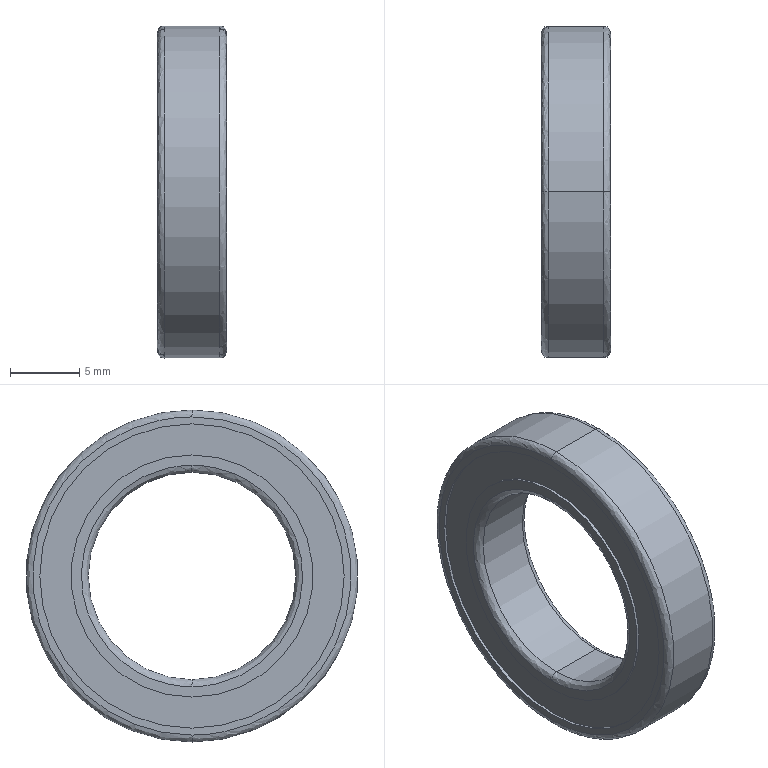Part | STEP file | Bearing 6802zz | 1 solid | 26 faces | box 5 x 24 x 24 mm | volume 1309 mm3 | cylinder 12 | spline 8 | plane 6 | commonest cylinder face diameters 17.5 x4 22 x4 15 x2 24 x2